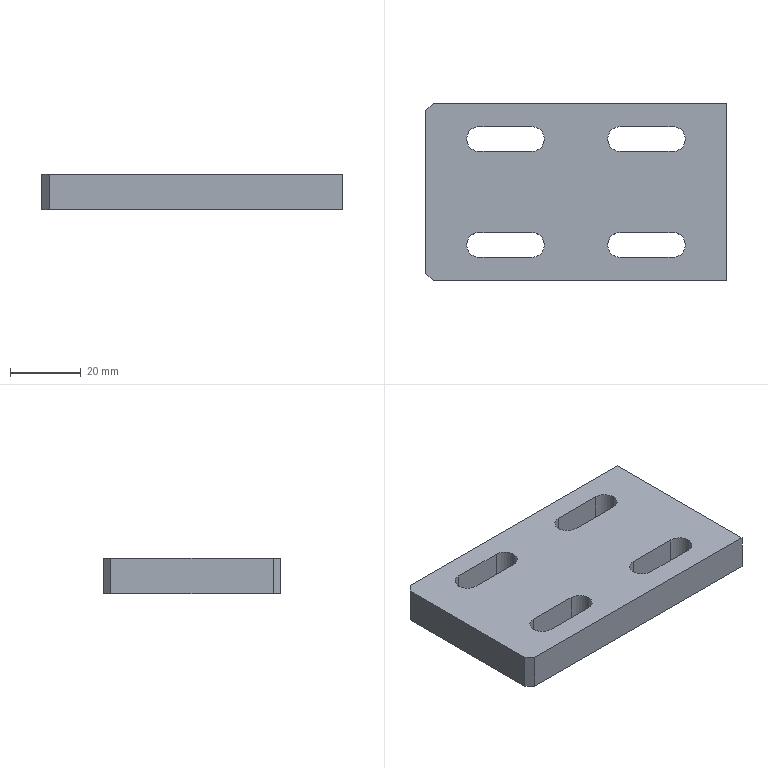Part | NX | 1 solid | 30 faces | box 85 x 50 x 10 mm | volume 36453 mm3 | plane 16 | cylinder 11 | cone 3 | commonest cylinder face diameters 7 x8 3.3 x3
STEP:
#1=CARTESIAN_POINT('',(-42.5,23.,-5.));
#2=VERTEX_POINT('',#1);
#3=CARTESIAN_POINT('',(-42.5,-23.,-5.));
#4=VERTEX_POINT('',#3);
#5=CARTESIAN_POINT('',(-42.5,-25.,-5.));
#6=DIRECTION('',(0.,-1.,0.));
#7=VECTOR('',#6,1000.);
#8=LINE('',#5,#7);
#9=EDGE_CURVE('',#2,#4,#8,.T.);
#10=ORIENTED_EDGE('',*,*,#9,.T.);
#11=CARTESIAN_POINT('',(-42.5,-23.,5.));
#12=VERTEX_POINT('',#11);
#13=CARTESIAN_POINT('',(-42.5,-23.,5.));
#14=DIRECTION('',(0.,0.,1.));
#15=VECTOR('',#14,1000.);
#16=LINE('',#13,#15);
#17=EDGE_CURVE('',#4,#12,#16,.T.);
#18=ORIENTED_EDGE('',*,*,#17,.T.);
#19=CARTESIAN_POINT('',(-42.5,23.,5.));
#20=VERTEX_POINT('',#19);
#21=CARTESIAN_POINT('',(-42.5,-25.,5.));
#22=DIRECTION('',(0.,-1.,0.));
#23=VECTOR('',#22,1000.);
#24=LINE('',#21,#23);
#25=EDGE_CURVE('',#20,#12,#24,.T.);
#26=ORIENTED_EDGE('',*,*,#25,.F.);
#27=CARTESIAN_POINT('',(-42.5,23.,5.));
#28=DIRECTION('',(0.,0.,-1.));
#29=VECTOR('',#28,1000.);
#30=LINE('',#27,#29);
#31=EDGE_CURVE('',#20,#2,#30,.T.);
#32=ORIENTED_EDGE('',*,*,#31,.T.);
#33=EDGE_LOOP('',(#10,#18,#26,#32));
#34=FACE_BOUND('',#33,.T.);
#35=CARTESIAN_POINT('',(-42.5,-25.,5.));
#36=DIRECTION('',(1.,0.,0.));
#37=DIRECTION('',(0.,0.,-1.));
#38=AXIS2_PLACEMENT_3D('',#35,#36,#37);
#39=PLANE('',#38);
#40=ADVANCED_FACE('',(#34),#39,.F.);
#41=CARTESIAN_POINT('',(-40.5,-25.,5.));
#42=VERTEX_POINT('',#41);
#43=CARTESIAN_POINT('',(42.5,-25.,5.));
#44=VERTEX_POINT('',#43);
#45=CARTESIAN_POINT('',(42.5,-25.,5.));
#46=DIRECTION('',(1.,0.,0.));
#47=VECTOR('',#46,1000.);
#48=LINE('',#45,#47);
#49=EDGE_CURVE('',#42,#44,#48,.T.);
#50=ORIENTED_EDGE('',*,*,#49,.F.);
#51=CARTESIAN_POINT('',(-40.5,-25.,-5.));
#52=VERTEX_POINT('',#51);
#53=CARTESIAN_POINT('',(-40.5,-25.,5.));
#54=DIRECTION('',(0.,0.,-1.));
#55=VECTOR('',#54,1000.);
#56=LINE('',#53,#55);
#57=EDGE_CURVE('',#42,#52,#56,.T.);
#58=ORIENTED_EDGE('',*,*,#57,.T.);
#59=CARTESIAN_POINT('',(42.5,-25.,-5.));
#60=VERTEX_POINT('',#59);
#61=CARTESIAN_POINT('',(42.5,-25.,-5.));
#62=DIRECTION('',(1.,0.,0.));
#63=VECTOR('',#62,1000.);
#64=LINE('',#61,#63);
#65=EDGE_CURVE('',#52,#60,#64,.T.);
#66=ORIENTED_EDGE('',*,*,#65,.T.);
#67=CARTESIAN_POINT('',(42.5,-25.,5.));
#68=DIRECTION('',(0.,0.,-1.));
#69=VECTOR('',#68,1000.);
#70=LINE('',#67,#69);
#71=EDGE_CURVE('',#44,#60,#70,.T.);
#72=ORIENTED_EDGE('',*,*,#71,.F.);
#73=EDGE_LOOP('',(#50,#58,#66,#72));
#74=FACE_BOUND('',#73,.T.);
#75=CARTESIAN_POINT('',(42.5,-25.,5.));
#76=DIRECTION('',(0.,1.,0.));
#77=DIRECTION('',(-1.,0.,0.));
#78=AXIS2_PLACEMENT_3D('',#75,#76,#77);
#79=PLANE('',#78);
#80=ADVANCED_FACE('',(#74),#79,.F.);
#81=CARTESIAN_POINT('',(42.5,17.5,-1.65));
#82=VERTEX_POINT('',#81);
#83=CARTESIAN_POINT('',(42.5,17.5,0.));
#84=DIRECTION('',(1.,0.,0.));
#85=DIRECTION('',(0.,0.,-1.));
#86=AXIS2_PLACEMENT_3D('',#83,#84,#85);
#87=CIRCLE('',#86,1.65);
#88=EDGE_CURVE('',#82,#82,#87,.T.);
#89=ORIENTED_EDGE('',*,*,#88,.F.);
#90=EDGE_LOOP('',(#89));
#91=FACE_BOUND('',#90,.T.);
#92=CARTESIAN_POINT('',(42.5,0.,-1.65));
#93=VERTEX_POINT('',#92);
#94=CARTESIAN_POINT('',(42.5,0.,0.));
#95=DIRECTION('',(1.,0.,0.));
#96=DIRECTION('',(0.,0.,-1.));
#97=AXIS2_PLACEMENT_3D('',#94,#95,#96);
#98=CIRCLE('',#97,1.65);
#99=EDGE_CURVE('',#93,#93,#98,.T.);
#100=ORIENTED_EDGE('',*,*,#99,.F.);
#101=EDGE_LOOP('',(#100));
#102=FACE_BOUND('',#101,.T.);
#103=CARTESIAN_POINT('',(42.5,-17.5,-1.65));
#104=VERTEX_POINT('',#103);
#105=CARTESIAN_POINT('',(42.5,-17.5,0.));
#106=DIRECTION('',(1.,0.,0.));
#107=DIRECTION('',(0.,0.,-1.));
#108=AXIS2_PLACEMENT_3D('',#105,#106,#107);
#109=CIRCLE('',#108,1.65);
#110=EDGE_CURVE('',#104,#104,#109,.T.);
#111=ORIENTED_EDGE('',*,*,#110,.F.);
#112=EDGE_LOOP('',(#111));
#113=FACE_BOUND('',#112,.T.);
#114=CARTESIAN_POINT('',(42.5,25.,-5.));
#115=VERTEX_POINT('',#114);
#116=CARTESIAN_POINT('',(42.5,-25.,-5.));
#117=DIRECTION('',(0.,1.,0.));
#118=VECTOR('',#117,1000.);
#119=LINE('',#116,#118);
#120=EDGE_CURVE('',#60,#115,#119,.T.);
#121=ORIENTED_EDGE('',*,*,#120,.T.);
#122=CARTESIAN_POINT('',(42.5,25.,5.));
#123=VERTEX_POINT('',#122);
#124=CARTESIAN_POINT('',(42.5,25.,5.));
#125=DIRECTION('',(0.,0.,-1.));
#126=VECTOR('',#125,1000.);
#127=LINE('',#124,#126);
#128=EDGE_CURVE('',#123,#115,#127,.T.);
#129=ORIENTED_EDGE('',*,*,#128,.F.);
#130=CARTESIAN_POINT('',(42.5,-25.,5.));
#131=DIRECTION('',(0.,1.,0.));
#132=VECTOR('',#131,1000.);
#133=LINE('',#130,#132);
#134=EDGE_CURVE('',#44,#123,#133,.T.);
#135=ORIENTED_EDGE('',*,*,#134,.F.);
#136=ORIENTED_EDGE('',*,*,#71,.T.);
#137=EDGE_LOOP('',(#121,#129,#135,#136));
#138=FACE_BOUND('',#137,.T.);
#139=CARTESIAN_POINT('',(42.5,-25.,5.));
#140=DIRECTION('',(-1.,0.,0.));
#141=DIRECTION('',(0.,0.,1.));
#142=AXIS2_PLACEMENT_3D('',#139,#140,#141);
#143=PLANE('',#142);
#144=ADVANCED_FACE('',(#91,#102,#113,#138),#143,.F.);
#145=CARTESIAN_POINT('',(-40.5,25.,-5.));
#146=VERTEX_POINT('',#145);
#147=CARTESIAN_POINT('',(42.5,25.,-5.));
#148=DIRECTION('',(-1.,0.,0.));
#149=VECTOR('',#148,1000.);
#150=LINE('',#147,#149);
#151=EDGE_CURVE('',#115,#146,#150,.T.);
#152=ORIENTED_EDGE('',*,*,#151,.T.);
#153=CARTESIAN_POINT('',(-40.5,25.,5.));
#154=VERTEX_POINT('',#153);
#155=CARTESIAN_POINT('',(-40.5,25.,5.));
#156=DIRECTION('',(0.,0.,1.));
#157=VECTOR('',#156,1000.);
#158=LINE('',#155,#157);
#159=EDGE_CURVE('',#146,#154,#158,.T.);
#160=ORIENTED_EDGE('',*,*,#159,.T.);
#161=CARTESIAN_POINT('',(42.5,25.,5.));
#162=DIRECTION('',(-1.,0.,0.));
#163=VECTOR('',#162,1000.);
#164=LINE('',#161,#163);
#165=EDGE_CURVE('',#123,#154,#164,.T.);
#166=ORIENTED_EDGE('',*,*,#165,.F.);
#167=ORIENTED_EDGE('',*,*,#128,.T.);
#168=EDGE_LOOP('',(#152,#160,#166,#167));
#169=FACE_BOUND('',#168,.T.);
#170=CARTESIAN_POINT('',(42.5,25.,5.));
#171=DIRECTION('',(0.,-1.,0.));
#172=DIRECTION('',(1.,0.,0.));
#173=AXIS2_PLACEMENT_3D('',#170,#171,#172);
#174=PLANE('',#173);
#175=ADVANCED_FACE('',(#169),#174,.F.);
#176=CARTESIAN_POINT('',(12.5,-11.5,5.));
#177=VERTEX_POINT('',#176);
#178=CARTESIAN_POINT('',(12.5,-18.5,5.));
#179=VERTEX_POINT('',#178);
#180=CARTESIAN_POINT('',(12.5,-15.,5.));
#181=DIRECTION('',(0.,0.,1.));
#182=DIRECTION('',(1.,0.,0.));
#183=AXIS2_PLACEMENT_3D('',#180,#181,#182);
#184=CIRCLE('',#183,3.5);
#185=EDGE_CURVE('',#177,#179,#184,.T.);
#186=ORIENTED_EDGE('',*,*,#185,.F.);
#187=CARTESIAN_POINT('',(27.5,-11.5,5.));
#188=VERTEX_POINT('',#187);
#189=CARTESIAN_POINT('',(12.5,-11.5,5.));
#190=DIRECTION('',(-1.,0.,0.));
#191=VECTOR('',#190,1000.);
#192=LINE('',#189,#191);
#193=EDGE_CURVE('',#188,#177,#192,.T.);
#194=ORIENTED_EDGE('',*,*,#193,.F.);
#195=CARTESIAN_POINT('',(27.5,-18.5,5.));
#196=VERTEX_POINT('',#195);
#197=CARTESIAN_POINT('',(27.5,-15.,5.));
#198=DIRECTION('',(0.,0.,1.));
#199=DIRECTION('',(1.,0.,0.));
#200=AXIS2_PLACEMENT_3D('',#197,#198,#199);
#201=CIRCLE('',#200,3.5);
#202=EDGE_CURVE('',#196,#188,#201,.T.);
#203=ORIENTED_EDGE('',*,*,#202,.F.);
#204=CARTESIAN_POINT('',(12.5,-18.5,5.));
#205=DIRECTION('',(1.,0.,0.));
#206=VECTOR('',#205,1000.);
#207=LINE('',#204,#206);
#208=EDGE_CURVE('',#179,#196,#207,.T.);
#209=ORIENTED_EDGE('',*,*,#208,.F.);
#210=EDGE_LOOP('',(#186,#194,#203,#209));
#211=FACE_BOUND('',#210,.T.);
#212=CARTESIAN_POINT('',(12.5,18.5,5.));
#213=VERTEX_POINT('',#212);
#214=CARTESIAN_POINT('',(12.5,11.5,5.));
#215=VERTEX_POINT('',#214);
#216=CARTESIAN_POINT('',(12.5,15.,5.));
#217=DIRECTION('',(0.,0.,1.));
#218=DIRECTION('',(1.,0.,0.));
#219=AXIS2_PLACEMENT_3D('',#216,#217,#218);
#220=CIRCLE('',#219,3.5);
#221=EDGE_CURVE('',#213,#215,#220,.T.);
#222=ORIENTED_EDGE('',*,*,#221,.F.);
#223=CARTESIAN_POINT('',(27.5,18.5,5.));
#224=VERTEX_POINT('',#223);
#225=CARTESIAN_POINT('',(12.5,18.5,5.));
#226=DIRECTION('',(-1.,0.,0.));
#227=VECTOR('',#226,1000.);
#228=LINE('',#225,#227);
#229=EDGE_CURVE('',#224,#213,#228,.T.);
#230=ORIENTED_EDGE('',*,*,#229,.F.);
#231=CARTESIAN_POINT('',(27.5,11.5,5.));
#232=VERTEX_POINT('',#231);
#233=CARTESIAN_POINT('',(27.5,15.,5.));
#234=DIRECTION('',(0.,0.,1.));
#235=DIRECTION('',(1.,0.,0.));
#236=AXIS2_PLACEMENT_3D('',#233,#234,#235);
#237=CIRCLE('',#236,3.5);
#238=EDGE_CURVE('',#232,#224,#237,.T.);
#239=ORIENTED_EDGE('',*,*,#238,.F.);
#240=CARTESIAN_POINT('',(12.5,11.5,5.));
#241=DIRECTION('',(1.,0.,0.));
#242=VECTOR('',#241,1000.);
#243=LINE('',#240,#242);
#244=EDGE_CURVE('',#215,#232,#243,.T.);
#245=ORIENTED_EDGE('',*,*,#244,.F.);
#246=EDGE_LOOP('',(#222,#230,#239,#245));
#247=FACE_BOUND('',#246,.T.);
#248=CARTESIAN_POINT('',(-27.5,-11.5,5.));
#249=VERTEX_POINT('',#248);
#250=CARTESIAN_POINT('',(-27.5,-18.5,5.));
#251=VERTEX_POINT('',#250);
#252=CARTESIAN_POINT('',(-27.5,-15.,5.));
#253=DIRECTION('',(0.,0.,1.));
#254=DIRECTION('',(1.,0.,0.));
#255=AXIS2_PLACEMENT_3D('',#252,#253,#254);
#256=CIRCLE('',#255,3.5);
#257=EDGE_CURVE('',#249,#251,#256,.T.);
#258=ORIENTED_EDGE('',*,*,#257,.F.);
#259=CARTESIAN_POINT('',(-12.5,-11.5,5.));
#260=VERTEX_POINT('',#259);
#261=CARTESIAN_POINT('',(-27.5,-11.5,5.));
#262=DIRECTION('',(-1.,0.,0.));
#263=VECTOR('',#262,1000.);
#264=LINE('',#261,#263);
#265=EDGE_CURVE('',#260,#249,#264,.T.);
#266=ORIENTED_EDGE('',*,*,#265,.F.);
#267=CARTESIAN_POINT('',(-12.5,-18.5,5.));
#268=VERTEX_POINT('',#267);
#269=CARTESIAN_POINT('',(-12.5,-15.,5.));
#270=DIRECTION('',(0.,0.,1.));
#271=DIRECTION('',(1.,0.,0.));
#272=AXIS2_PLACEMENT_3D('',#269,#270,#271);
#273=CIRCLE('',#272,3.5);
#274=EDGE_CURVE('',#268,#260,#273,.T.);
#275=ORIENTED_EDGE('',*,*,#274,.F.);
#276=CARTESIAN_POINT('',(-27.5,-18.5,5.));
#277=DIRECTION('',(1.,0.,0.));
#278=VECTOR('',#277,1000.);
#279=LINE('',#276,#278);
#280=EDGE_CURVE('',#251,#268,#279,.T.);
#281=ORIENTED_EDGE('',*,*,#280,.F.);
#282=EDGE_LOOP('',(#258,#266,#275,#281));
#283=FACE_BOUND('',#282,.T.);
#284=CARTESIAN_POINT('',(-27.5,18.5,5.));
#285=VERTEX_POINT('',#284);
#286=CARTESIAN_POINT('',(-27.5,11.5,5.));
#287=VERTEX_POINT('',#286);
#288=CARTESIAN_POINT('',(-27.5,15.,5.));
#289=DIRECTION('',(0.,0.,1.));
#290=DIRECTION('',(1.,0.,0.));
#291=AXIS2_PLACEMENT_3D('',#288,#289,#290);
#292=CIRCLE('',#291,3.5);
#293=EDGE_CURVE('',#285,#287,#292,.T.);
#294=ORIENTED_EDGE('',*,*,#293,.F.);
#295=CARTESIAN_POINT('',(-12.5,18.5,5.));
#296=VERTEX_POINT('',#295);
#297=CARTESIAN_POINT('',(-27.5,18.5,5.));
#298=DIRECTION('',(-1.,0.,0.));
#299=VECTOR('',#298,1000.);
#300=LINE('',#297,#299);
#301=EDGE_CURVE('',#296,#285,#300,.T.);
#302=ORIENTED_EDGE('',*,*,#301,.F.);
#303=CARTESIAN_POINT('',(-12.5,11.5,5.));
#304=VERTEX_POINT('',#303);
#305=CARTESIAN_POINT('',(-12.5,15.,5.));
#306=DIRECTION('',(0.,0.,1.));
#307=DIRECTION('',(1.,0.,0.));
#308=AXIS2_PLACEMENT_3D('',#305,#306,#307);
#309=CIRCLE('',#308,3.5);
#310=EDGE_CURVE('',#304,#296,#309,.T.);
#311=ORIENTED_EDGE('',*,*,#310,.F.);
#312=CARTESIAN_POINT('',(-27.5,11.5,5.));
#313=DIRECTION('',(1.,0.,0.));
#314=VECTOR('',#313,1000.);
#315=LINE('',#312,#314);
#316=EDGE_CURVE('',#287,#304,#315,.T.);
#317=ORIENTED_EDGE('',*,*,#316,.F.);
#318=EDGE_LOOP('',(#294,#302,#311,#317));
#319=FACE_BOUND('',#318,.T.);
#320=ORIENTED_EDGE('',*,*,#25,.T.);
#321=CARTESIAN_POINT('',(-32.75,-32.75,5.));
#322=DIRECTION('',(-0.7071,0.7071,0.));
#323=VECTOR('',#322,1000.);
#324=LINE('',#321,#323);
#325=EDGE_CURVE('',#12,#42,#324,.F.);
#326=ORIENTED_EDGE('',*,*,#325,.T.);
#327=ORIENTED_EDGE('',*,*,#49,.T.);
#328=ORIENTED_EDGE('',*,*,#134,.T.);
#329=ORIENTED_EDGE('',*,*,#165,.T.);
#330=CARTESIAN_POINT('',(-32.75,32.75,5.));
#331=DIRECTION('',(0.7071,0.7071,0.));
#332=VECTOR('',#331,1000.);
#333=LINE('',#330,#332);
#334=EDGE_CURVE('',#154,#20,#333,.F.);
#335=ORIENTED_EDGE('',*,*,#334,.T.);
#336=EDGE_LOOP('',(#320,#326,#327,#328,#329,#335));
#337=FACE_BOUND('',#336,.T.);
#338=CARTESIAN_POINT('',(0.,0.,5.));
#339=DIRECTION('',(0.,0.,1.));
#340=DIRECTION('',(1.,0.,0.));
#341=AXIS2_PLACEMENT_3D('',#338,#339,#340);
#342=PLANE('',#341);
#343=ADVANCED_FACE('',(#211,#247,#283,#319,#337),#342,.T.);
#344=CARTESIAN_POINT('',(27.5,-11.5,-5.));
#345=VERTEX_POINT('',#344);
#346=CARTESIAN_POINT('',(12.5,-11.5,-5.));
#347=VERTEX_POINT('',#346);
#348=CARTESIAN_POINT('',(12.5,-11.5,-5.));
#349=DIRECTION('',(-1.,0.,0.));
#350=VECTOR('',#349,1000.);
#351=LINE('',#348,#350);
#352=EDGE_CURVE('',#345,#347,#351,.T.);
#353=ORIENTED_EDGE('',*,*,#352,.T.);
#354=CARTESIAN_POINT('',(12.5,-18.5,-5.));
#355=VERTEX_POINT('',#354);
#356=CARTESIAN_POINT('',(12.5,-15.,-5.));
#357=DIRECTION('',(0.,0.,1.));
#358=DIRECTION('',(1.,0.,0.));
#359=AXIS2_PLACEMENT_3D('',#356,#357,#358);
#360=CIRCLE('',#359,3.5);
#361=EDGE_CURVE('',#347,#355,#360,.T.);
#362=ORIENTED_EDGE('',*,*,#361,.T.);
#363=CARTESIAN_POINT('',(27.5,-18.5,-5.));
#364=VERTEX_POINT('',#363);
#365=CARTESIAN_POINT('',(12.5,-18.5,-5.));
#366=DIRECTION('',(1.,0.,0.));
#367=VECTOR('',#366,1000.);
#368=LINE('',#365,#367);
#369=EDGE_CURVE('',#355,#364,#368,.T.);
#370=ORIENTED_EDGE('',*,*,#369,.T.);
#371=CARTESIAN_POINT('',(27.5,-15.,-5.));
#372=DIRECTION('',(0.,0.,1.));
#373=DIRECTION('',(1.,0.,0.));
#374=AXIS2_PLACEMENT_3D('',#371,#372,#373);
#375=CIRCLE('',#374,3.5);
#376=EDGE_CURVE('',#364,#345,#375,.T.);
#377=ORIENTED_EDGE('',*,*,#376,.T.);
#378=EDGE_LOOP('',(#353,#362,#370,#377));
#379=FACE_BOUND('',#378,.T.);
#380=CARTESIAN_POINT('',(27.5,18.5,-5.));
#381=VERTEX_POINT('',#380);
#382=CARTESIAN_POINT('',(12.5,18.5,-5.));
#383=VERTEX_POINT('',#382);
#384=CARTESIAN_POINT('',(12.5,18.5,-5.));
#385=DIRECTION('',(-1.,0.,0.));
#386=VECTOR('',#385,1000.);
#387=LINE('',#384,#386);
#388=EDGE_CURVE('',#381,#383,#387,.T.);
#389=ORIENTED_EDGE('',*,*,#388,.T.);
#390=CARTESIAN_POINT('',(12.5,11.5,-5.));
#391=VERTEX_POINT('',#390);
#392=CARTESIAN_POINT('',(12.5,15.,-5.));
#393=DIRECTION('',(0.,0.,1.));
#394=DIRECTION('',(1.,0.,0.));
#395=AXIS2_PLACEMENT_3D('',#392,#393,#394);
#396=CIRCLE('',#395,3.5);
#397=EDGE_CURVE('',#383,#391,#396,.T.);
#398=ORIENTED_EDGE('',*,*,#397,.T.);
#399=CARTESIAN_POINT('',(27.5,11.5,-5.));
#400=VERTEX_POINT('',#399);
#401=CARTESIAN_POINT('',(12.5,11.5,-5.));
#402=DIRECTION('',(1.,0.,0.));
#403=VECTOR('',#402,1000.);
#404=LINE('',#401,#403);
#405=EDGE_CURVE('',#391,#400,#404,.T.);
#406=ORIENTED_EDGE('',*,*,#405,.T.);
#407=CARTESIAN_POINT('',(27.5,15.,-5.));
#408=DIRECTION('',(0.,0.,1.));
#409=DIRECTION('',(1.,0.,0.));
#410=AXIS2_PLACEMENT_3D('',#407,#408,#409);
#411=CIRCLE('',#410,3.5);
#412=EDGE_CURVE('',#400,#381,#411,.T.);
#413=ORIENTED_EDGE('',*,*,#412,.T.);
#414=EDGE_LOOP('',(#389,#398,#406,#413));
#415=FACE_BOUND('',#414,.T.);
#416=CARTESIAN_POINT('',(-12.5,-11.5,-5.));
#417=VERTEX_POINT('',#416);
#418=CARTESIAN_POINT('',(-27.5,-11.5,-5.));
#419=VERTEX_POINT('',#418);
#420=CARTESIAN_POINT('',(-27.5,-11.5,-5.));
#421=DIRECTION('',(-1.,0.,0.));
#422=VECTOR('',#421,1000.);
#423=LINE('',#420,#422);
#424=EDGE_CURVE('',#417,#419,#423,.T.);
#425=ORIENTED_EDGE('',*,*,#424,.T.);
#426=CARTESIAN_POINT('',(-27.5,-18.5,-5.));
#427=VERTEX_POINT('',#426);
#428=CARTESIAN_POINT('',(-27.5,-15.,-5.));
#429=DIRECTION('',(0.,0.,1.));
#430=DIRECTION('',(1.,0.,0.));
#431=AXIS2_PLACEMENT_3D('',#428,#429,#430);
#432=CIRCLE('',#431,3.5);
#433=EDGE_CURVE('',#419,#427,#432,.T.);
#434=ORIENTED_EDGE('',*,*,#433,.T.);
#435=CARTESIAN_POINT('',(-12.5,-18.5,-5.));
#436=VERTEX_POINT('',#435);
#437=CARTESIAN_POINT('',(-27.5,-18.5,-5.));
#438=DIRECTION('',(1.,0.,0.));
#439=VECTOR('',#438,1000.);
#440=LINE('',#437,#439);
#441=EDGE_CURVE('',#427,#436,#440,.T.);
#442=ORIENTED_EDGE('',*,*,#441,.T.);
#443=CARTESIAN_POINT('',(-12.5,-15.,-5.));
#444=DIRECTION('',(0.,0.,1.));
#445=DIRECTION('',(1.,0.,0.));
#446=AXIS2_PLACEMENT_3D('',#443,#444,#445);
#447=CIRCLE('',#446,3.5);
#448=EDGE_CURVE('',#436,#417,#447,.T.);
#449=ORIENTED_EDGE('',*,*,#448,.T.);
#450=EDGE_LOOP('',(#425,#434,#442,#449));
#451=FACE_BOUND('',#450,.T.);
#452=CARTESIAN_POINT('',(-12.5,18.5,-5.));
#453=VERTEX_POINT('',#452);
#454=CARTESIAN_POINT('',(-27.5,18.5,-5.));
#455=VERTEX_POINT('',#454);
#456=CARTESIAN_POINT('',(-27.5,18.5,-5.));
#457=DIRECTION('',(-1.,0.,0.));
#458=VECTOR('',#457,1000.);
#459=LINE('',#456,#458);
#460=EDGE_CURVE('',#453,#455,#459,.T.);
#461=ORIENTED_EDGE('',*,*,#460,.T.);
#462=CARTESIAN_POINT('',(-27.5,11.5,-5.));
#463=VERTEX_POINT('',#462);
#464=CARTESIAN_POINT('',(-27.5,15.,-5.));
#465=DIRECTION('',(0.,0.,1.));
#466=DIRECTION('',(1.,0.,0.));
#467=AXIS2_PLACEMENT_3D('',#464,#465,#466);
#468=CIRCLE('',#467,3.5);
#469=EDGE_CURVE('',#455,#463,#468,.T.);
#470=ORIENTED_EDGE('',*,*,#469,.T.);
#471=CARTESIAN_POINT('',(-12.5,11.5,-5.));
#472=VERTEX_POINT('',#471);
#473=CARTESIAN_POINT('',(-27.5,11.5,-5.));
#474=DIRECTION('',(1.,0.,0.));
#475=VECTOR('',#474,1000.);
#476=LINE('',#473,#475);
#477=EDGE_CURVE('',#463,#472,#476,.T.);
#478=ORIENTED_EDGE('',*,*,#477,.T.);
#479=CARTESIAN_POINT('',(-12.5,15.,-5.));
#480=DIRECTION('',(0.,0.,1.));
#481=DIRECTION('',(1.,0.,0.));
#482=AXIS2_PLACEMENT_3D('',#479,#480,#481);
#483=CIRCLE('',#482,3.5);
#484=EDGE_CURVE('',#472,#453,#483,.T.);
#485=ORIENTED_EDGE('',*,*,#484,.T.);
#486=EDGE_LOOP('',(#461,#470,#478,#485));
#487=FACE_BOUND('',#486,.T.);
#488=ORIENTED_EDGE('',*,*,#65,.F.);
#489=CARTESIAN_POINT('',(-40.5,-25.,-5.));
#490=DIRECTION('',(0.7071,-0.7071,0.));
#491=VECTOR('',#490,1000.);
#492=LINE('',#489,#491);
#493=EDGE_CURVE('',#52,#4,#492,.F.);
#494=ORIENTED_EDGE('',*,*,#493,.T.);
#495=ORIENTED_EDGE('',*,*,#9,.F.);
#496=CARTESIAN_POINT('',(-42.5,23.,-5.));
#497=DIRECTION('',(-0.7071,-0.7071,0.));
#498=VECTOR('',#497,1000.);
#499=LINE('',#496,#498);
#500=EDGE_CURVE('',#2,#146,#499,.F.);
#501=ORIENTED_EDGE('',*,*,#500,.T.);
#502=ORIENTED_EDGE('',*,*,#151,.F.);
#503=ORIENTED_EDGE('',*,*,#120,.F.);
#504=EDGE_LOOP('',(#488,#494,#495,#501,#502,#503));
#505=FACE_BOUND('',#504,.T.);
#506=CARTESIAN_POINT('',(0.,0.,-5.));
#507=DIRECTION('',(0.,0.,1.));
#508=DIRECTION('',(1.,0.,0.));
#509=AXIS2_PLACEMENT_3D('',#506,#507,#508);
#510=PLANE('',#509);
#511=ADVANCED_FACE('',(#379,#415,#451,#487,#505),#510,.F.);
#512=ORIENTED_EDGE('',*,*,#293,.T.);
#513=CARTESIAN_POINT('',(-27.5,11.5,-5.));
#514=DIRECTION('',(0.,0.,1.));
#515=VECTOR('',#514,1000.);
#516=LINE('',#513,#515);
#517=EDGE_CURVE('',#463,#287,#516,.T.);
#518=ORIENTED_EDGE('',*,*,#517,.F.);
#519=ORIENTED_EDGE('',*,*,#469,.F.);
#520=CARTESIAN_POINT('',(-27.5,18.5,-5.));
#521=DIRECTION('',(0.,0.,1.));
#522=VECTOR('',#521,1000.);
#523=LINE('',#520,#522);
#524=EDGE_CURVE('',#455,#285,#523,.T.);
#525=ORIENTED_EDGE('',*,*,#524,.T.);
#526=EDGE_LOOP('',(#512,#518,#519,#525));
#527=FACE_BOUND('',#526,.T.);
#528=CARTESIAN_POINT('',(-27.5,15.,-5.));
#529=DIRECTION('',(0.,0.,1.));
#530=DIRECTION('',(1.,0.,0.));
#531=AXIS2_PLACEMENT_3D('',#528,#529,#530);
#532=CYLINDRICAL_SURFACE('',#531,3.5);
#533=ADVANCED_FACE('',(#527),#532,.F.);
#534=ORIENTED_EDGE('',*,*,#301,.T.);
#535=ORIENTED_EDGE('',*,*,#524,.F.);
#536=ORIENTED_EDGE('',*,*,#460,.F.);
#537=CARTESIAN_POINT('',(-12.5,18.5,-5.));
#538=DIRECTION('',(0.,0.,1.));
#539=VECTOR('',#538,1000.);
#540=LINE('',#537,#539);
#541=EDGE_CURVE('',#453,#296,#540,.T.);
#542=ORIENTED_EDGE('',*,*,#541,.T.);
#543=EDGE_LOOP('',(#534,#535,#536,#542));
#544=FACE_BOUND('',#543,.T.);
#545=CARTESIAN_POINT('',(-27.5,18.5,-5.));
#546=DIRECTION('',(0.,1.,0.));
#547=DIRECTION('',(-1.,0.,0.));
#548=AXIS2_PLACEMENT_3D('',#545,#546,#547);
#549=PLANE('',#548);
#550=ADVANCED_FACE('',(#544),#549,.F.);
#551=ORIENTED_EDGE('',*,*,#310,.T.);
#552=ORIENTED_EDGE('',*,*,#541,.F.);
#553=ORIENTED_EDGE('',*,*,#484,.F.);
#554=CARTESIAN_POINT('',(-12.5,11.5,-5.));
#555=DIRECTION('',(0.,0.,1.));
#556=VECTOR('',#555,1000.);
#557=LINE('',#554,#556);
#558=EDGE_CURVE('',#472,#304,#557,.T.);
#559=ORIENTED_EDGE('',*,*,#558,.T.);
#560=EDGE_LOOP('',(#551,#552,#553,#559));
#561=FACE_BOUND('',#560,.T.);
#562=CARTESIAN_POINT('',(-12.5,15.,-5.));
#563=DIRECTION('',(0.,0.,1.));
#564=DIRECTION('',(1.,0.,0.));
#565=AXIS2_PLACEMENT_3D('',#562,#563,#564);
#566=CYLINDRICAL_SURFACE('',#565,3.5);
#567=ADVANCED_FACE('',(#561),#566,.F.);
#568=ORIENTED_EDGE('',*,*,#316,.T.);
#569=ORIENTED_EDGE('',*,*,#558,.F.);
#570=ORIENTED_EDGE('',*,*,#477,.F.);
#571=ORIENTED_EDGE('',*,*,#517,.T.);
#572=EDGE_LOOP('',(#568,#569,#570,#571));
#573=FACE_BOUND('',#572,.T.);
#574=CARTESIAN_POINT('',(-27.5,11.5,-5.));
#575=DIRECTION('',(0.,-1.,0.));
#576=DIRECTION('',(1.,0.,0.));
#577=AXIS2_PLACEMENT_3D('',#574,#575,#576);
#578=PLANE('',#577);
#579=ADVANCED_FACE('',(#573),#578,.F.);
#580=ORIENTED_EDGE('',*,*,#257,.T.);
#581=CARTESIAN_POINT('',(-27.5,-18.5,-5.));
#582=DIRECTION('',(0.,0.,1.));
#583=VECTOR('',#582,1000.);
#584=LINE('',#581,#583);
#585=EDGE_CURVE('',#427,#251,#584,.T.);
#586=ORIENTED_EDGE('',*,*,#585,.F.);
#587=ORIENTED_EDGE('',*,*,#433,.F.);
#588=CARTESIAN_POINT('',(-27.5,-11.5,-5.));
#589=DIRECTION('',(0.,0.,1.));
#590=VECTOR('',#589,1000.);
#591=LINE('',#588,#590);
#592=EDGE_CURVE('',#419,#249,#591,.T.);
#593=ORIENTED_EDGE('',*,*,#592,.T.);
#594=EDGE_LOOP('',(#580,#586,#587,#593));
#595=FACE_BOUND('',#594,.T.);
#596=CARTESIAN_POINT('',(-27.5,-15.,-5.));
#597=DIRECTION('',(0.,0.,1.));
#598=DIRECTION('',(1.,0.,0.));
#599=AXIS2_PLACEMENT_3D('',#596,#597,#598);
#600=CYLINDRICAL_SURFACE('',#599,3.5);
#601=ADVANCED_FACE('',(#595),#600,.F.);
#602=ORIENTED_EDGE('',*,*,#265,.T.);
#603=ORIENTED_EDGE('',*,*,#592,.F.);
#604=ORIENTED_EDGE('',*,*,#424,.F.);
#605=CARTESIAN_POINT('',(-12.5,-11.5,-5.));
#606=DIRECTION('',(0.,0.,1.));
#607=VECTOR('',#606,1000.);
#608=LINE('',#605,#607);
#609=EDGE_CURVE('',#417,#260,#608,.T.);
#610=ORIENTED_EDGE('',*,*,#609,.T.);
#611=EDGE_LOOP('',(#602,#603,#604,#610));
#612=FACE_BOUND('',#611,.T.);
#613=CARTESIAN_POINT('',(-27.5,-11.5,-5.));
#614=DIRECTION('',(0.,1.,0.));
#615=DIRECTION('',(-1.,0.,0.));
#616=AXIS2_PLACEMENT_3D('',#613,#614,#615);
#617=PLANE('',#616);
#618=ADVANCED_FACE('',(#612),#617,.F.);
#619=ORIENTED_EDGE('',*,*,#274,.T.);
#620=ORIENTED_EDGE('',*,*,#609,.F.);
#621=ORIENTED_EDGE('',*,*,#448,.F.);
#622=CARTESIAN_POINT('',(-12.5,-18.5,-5.));
#623=DIRECTION('',(0.,0.,1.));
#624=VECTOR('',#623,1000.);
#625=LINE('',#622,#624);
#626=EDGE_CURVE('',#436,#268,#625,.T.);
#627=ORIENTED_EDGE('',*,*,#626,.T.);
#628=EDGE_LOOP('',(#619,#620,#621,#627));
#629=FACE_BOUND('',#628,.T.);
#630=CARTESIAN_POINT('',(-12.5,-15.,-5.));
#631=DIRECTION('',(0.,0.,1.));
#632=DIRECTION('',(1.,0.,0.));
#633=AXIS2_PLACEMENT_3D('',#630,#631,#632);
#634=CYLINDRICAL_SURFACE('',#633,3.5);
#635=ADVANCED_FACE('',(#629),#634,.F.);
#636=ORIENTED_EDGE('',*,*,#280,.T.);
#637=ORIENTED_EDGE('',*,*,#626,.F.);
#638=ORIENTED_EDGE('',*,*,#441,.F.);
#639=ORIENTED_EDGE('',*,*,#585,.T.);
#640=EDGE_LOOP('',(#636,#637,#638,#639));
#641=FACE_BOUND('',#640,.T.);
#642=CARTESIAN_POINT('',(-27.5,-18.5,-5.));
#643=DIRECTION('',(0.,-1.,0.));
#644=DIRECTION('',(1.,0.,0.));
#645=AXIS2_PLACEMENT_3D('',#642,#643,#644);
#646=PLANE('',#645);
#647=ADVANCED_FACE('',(#641),#646,.F.);
#648=CARTESIAN_POINT('',(31.409,-17.5,0.));
#649=VERTEX_POINT('',#648);
#650=VERTEX_LOOP('',#649);
#651=FACE_BOUND('',#650,.T.);
#652=CARTESIAN_POINT('',(32.4,-17.5,-1.65));
#653=VERTEX_POINT('',#652);
#654=CARTESIAN_POINT('',(32.4,-17.5,0.));
#655=DIRECTION('',(1.,0.,0.));
#656=DIRECTION('',(0.,0.,-1.));
#657=AXIS2_PLACEMENT_3D('',#654,#655,#656);
#658=CIRCLE('',#657,1.65);
#659=EDGE_CURVE('',#653,#653,#658,.T.);
#660=ORIENTED_EDGE('',*,*,#659,.T.);
#661=EDGE_LOOP('',(#660));
#662=FACE_BOUND('',#661,.T.);
#663=CARTESIAN_POINT('',(32.4,-17.5,0.));
#664=DIRECTION('',(1.,0.,0.));
#665=DIRECTION('',(0.,0.,-1.));
#666=AXIS2_PLACEMENT_3D('',#663,#664,#665);
#667=CONICAL_SURFACE('',#666,1.65,1.03);
#668=ADVANCED_FACE('',(#651,#662),#667,.F.);
#669=ORIENTED_EDGE('',*,*,#659,.F.);
#670=EDGE_LOOP('',(#669));
#671=FACE_BOUND('',#670,.T.);
#672=ORIENTED_EDGE('',*,*,#110,.T.);
#673=EDGE_LOOP('',(#672));
#674=FACE_BOUND('',#673,.T.);
#675=CARTESIAN_POINT('',(42.5,-17.5,0.));
#676=DIRECTION('',(1.,0.,0.));
#677=DIRECTION('',(0.,0.,-1.));
#678=AXIS2_PLACEMENT_3D('',#675,#676,#677);
#679=CYLINDRICAL_SURFACE('',#678,1.65);
#680=ADVANCED_FACE('',(#671,#674),#679,.F.);
#681=CARTESIAN_POINT('',(31.409,0.,0.));
#682=VERTEX_POINT('',#681);
#683=VERTEX_LOOP('',#682);
#684=FACE_BOUND('',#683,.T.);
#685=CARTESIAN_POINT('',(32.4,0.,-1.65));
#686=VERTEX_POINT('',#685);
#687=CARTESIAN_POINT('',(32.4,0.,0.));
#688=DIRECTION('',(1.,0.,0.));
#689=DIRECTION('',(0.,0.,-1.));
#690=AXIS2_PLACEMENT_3D('',#687,#688,#689);
#691=CIRCLE('',#690,1.65);
#692=EDGE_CURVE('',#686,#686,#691,.T.);
#693=ORIENTED_EDGE('',*,*,#692,.T.);
#694=EDGE_LOOP('',(#693));
#695=FACE_BOUND('',#694,.T.);
#696=CARTESIAN_POINT('',(32.4,0.,0.));
#697=DIRECTION('',(1.,0.,0.));
#698=DIRECTION('',(0.,0.,-1.));
#699=AXIS2_PLACEMENT_3D('',#696,#697,#698);
#700=CONICAL_SURFACE('',#699,1.65,1.03);
#701=ADVANCED_FACE('',(#684,#695),#700,.F.);
#702=ORIENTED_EDGE('',*,*,#692,.F.);
#703=EDGE_LOOP('',(#702));
#704=FACE_BOUND('',#703,.T.);
#705=ORIENTED_EDGE('',*,*,#99,.T.);
#706=EDGE_LOOP('',(#705));
#707=FACE_BOUND('',#706,.T.);
#708=CARTESIAN_POINT('',(42.5,0.,0.));
#709=DIRECTION('',(1.,0.,0.));
#710=DIRECTION('',(0.,0.,-1.));
#711=AXIS2_PLACEMENT_3D('',#708,#709,#710);
#712=CYLINDRICAL_SURFACE('',#711,1.65);
#713=ADVANCED_FACE('',(#704,#707),#712,.F.);
#714=CARTESIAN_POINT('',(31.409,17.5,0.));
#715=VERTEX_POINT('',#714);
#716=VERTEX_LOOP('',#715);
#717=FACE_BOUND('',#716,.T.);
#718=CARTESIAN_POINT('',(32.4,17.5,-1.65));
#719=VERTEX_POINT('',#718);
#720=CARTESIAN_POINT('',(32.4,17.5,0.));
#721=DIRECTION('',(1.,0.,0.));
#722=DIRECTION('',(0.,0.,-1.));
#723=AXIS2_PLACEMENT_3D('',#720,#721,#722);
#724=CIRCLE('',#723,1.65);
#725=EDGE_CURVE('',#719,#719,#724,.T.);
#726=ORIENTED_EDGE('',*,*,#725,.T.);
#727=EDGE_LOOP('',(#726));
#728=FACE_BOUND('',#727,.T.);
#729=CARTESIAN_POINT('',(32.4,17.5,0.));
#730=DIRECTION('',(1.,0.,0.));
#731=DIRECTION('',(0.,0.,-1.));
#732=AXIS2_PLACEMENT_3D('',#729,#730,#731);
#733=CONICAL_SURFACE('',#732,1.65,1.03);
#734=ADVANCED_FACE('',(#717,#728),#733,.F.);
#735=ORIENTED_EDGE('',*,*,#725,.F.);
#736=EDGE_LOOP('',(#735));
#737=FACE_BOUND('',#736,.T.);
#738=ORIENTED_EDGE('',*,*,#88,.T.);
#739=EDGE_LOOP('',(#738));
#740=FACE_BOUND('',#739,.T.);
#741=CARTESIAN_POINT('',(42.5,17.5,0.));
#742=DIRECTION('',(1.,0.,0.));
#743=DIRECTION('',(0.,0.,-1.));
#744=AXIS2_PLACEMENT_3D('',#741,#742,#743);
#745=CYLINDRICAL_SURFACE('',#744,1.65);
#746=ADVANCED_FACE('',(#737,#740),#745,.F.);
#747=ORIENTED_EDGE('',*,*,#325,.F.);
#748=ORIENTED_EDGE('',*,*,#17,.F.);
#749=ORIENTED_EDGE('',*,*,#493,.F.);
#750=ORIENTED_EDGE('',*,*,#57,.F.);
#751=EDGE_LOOP('',(#747,#748,#749,#750));
#752=FACE_BOUND('',#751,.T.);
#753=CARTESIAN_POINT('',(-40.5,-25.,5.));
#754=DIRECTION('',(0.7071,0.7071,0.));
#755=DIRECTION('',(0.,0.,-1.));
#756=AXIS2_PLACEMENT_3D('',#753,#754,#755);
#757=PLANE('',#756);
#758=ADVANCED_FACE('',(#752),#757,.F.);
#759=ORIENTED_EDGE('',*,*,#334,.F.);
#760=ORIENTED_EDGE('',*,*,#159,.F.);
#761=ORIENTED_EDGE('',*,*,#500,.F.);
#762=ORIENTED_EDGE('',*,*,#31,.F.);
#763=EDGE_LOOP('',(#759,#760,#761,#762));
#764=FACE_BOUND('',#763,.T.);
#765=CARTESIAN_POINT('',(-42.5,23.,5.));
#766=DIRECTION('',(0.7071,-0.7071,0.));
#767=DIRECTION('',(0.,0.,-1.));
#768=AXIS2_PLACEMENT_3D('',#765,#766,#767);
#769=PLANE('',#768);
#770=ADVANCED_FACE('',(#764),#769,.F.);
#771=ORIENTED_EDGE('',*,*,#221,.T.);
#772=CARTESIAN_POINT('',(12.5,11.5,-5.));
#773=DIRECTION('',(0.,0.,1.));
#774=VECTOR('',#773,1000.);
#775=LINE('',#772,#774);
#776=EDGE_CURVE('',#391,#215,#775,.T.);
#777=ORIENTED_EDGE('',*,*,#776,.F.);
#778=ORIENTED_EDGE('',*,*,#397,.F.);
#779=CARTESIAN_POINT('',(12.5,18.5,-5.));
#780=DIRECTION('',(0.,0.,1.));
#781=VECTOR('',#780,1000.);
#782=LINE('',#779,#781);
#783=EDGE_CURVE('',#383,#213,#782,.T.);
#784=ORIENTED_EDGE('',*,*,#783,.T.);
#785=EDGE_LOOP('',(#771,#777,#778,#784));
#786=FACE_BOUND('',#785,.T.);
#787=CARTESIAN_POINT('',(12.5,15.,-5.));
#788=DIRECTION('',(0.,0.,1.));
#789=DIRECTION('',(1.,0.,0.));
#790=AXIS2_PLACEMENT_3D('',#787,#788,#789);
#791=CYLINDRICAL_SURFACE('',#790,3.5);
#792=ADVANCED_FACE('',(#786),#791,.F.);
#793=ORIENTED_EDGE('',*,*,#229,.T.);
#794=ORIENTED_EDGE('',*,*,#783,.F.);
#795=ORIENTED_EDGE('',*,*,#388,.F.);
#796=CARTESIAN_POINT('',(27.5,18.5,-5.));
#797=DIRECTION('',(0.,0.,1.));
#798=VECTOR('',#797,1000.);
#799=LINE('',#796,#798);
#800=EDGE_CURVE('',#381,#224,#799,.T.);
#801=ORIENTED_EDGE('',*,*,#800,.T.);
#802=EDGE_LOOP('',(#793,#794,#795,#801));
#803=FACE_BOUND('',#802,.T.);
#804=CARTESIAN_POINT('',(12.5,18.5,-5.));
#805=DIRECTION('',(0.,1.,0.));
#806=DIRECTION('',(-1.,0.,0.));
#807=AXIS2_PLACEMENT_3D('',#804,#805,#806);
#808=PLANE('',#807);
#809=ADVANCED_FACE('',(#803),#808,.F.);
#810=ORIENTED_EDGE('',*,*,#238,.T.);
#811=ORIENTED_EDGE('',*,*,#800,.F.);
#812=ORIENTED_EDGE('',*,*,#412,.F.);
#813=CARTESIAN_POINT('',(27.5,11.5,-5.));
#814=DIRECTION('',(0.,0.,1.));
#815=VECTOR('',#814,1000.);
#816=LINE('',#813,#815);
#817=EDGE_CURVE('',#400,#232,#816,.T.);
#818=ORIENTED_EDGE('',*,*,#817,.T.);
#819=EDGE_LOOP('',(#810,#811,#812,#818));
#820=FACE_BOUND('',#819,.T.);
#821=CARTESIAN_POINT('',(27.5,15.,-5.));
#822=DIRECTION('',(0.,0.,1.));
#823=DIRECTION('',(1.,0.,0.));
#824=AXIS2_PLACEMENT_3D('',#821,#822,#823);
#825=CYLINDRICAL_SURFACE('',#824,3.5);
#826=ADVANCED_FACE('',(#820),#825,.F.);
#827=ORIENTED_EDGE('',*,*,#244,.T.);
#828=ORIENTED_EDGE('',*,*,#817,.F.);
#829=ORIENTED_EDGE('',*,*,#405,.F.);
#830=ORIENTED_EDGE('',*,*,#776,.T.);
#831=EDGE_LOOP('',(#827,#828,#829,#830));
#832=FACE_BOUND('',#831,.T.);
#833=CARTESIAN_POINT('',(12.5,11.5,-5.));
#834=DIRECTION('',(0.,-1.,0.));
#835=DIRECTION('',(1.,0.,0.));
#836=AXIS2_PLACEMENT_3D('',#833,#834,#835);
#837=PLANE('',#836);
#838=ADVANCED_FACE('',(#832),#837,.F.);
#839=ORIENTED_EDGE('',*,*,#185,.T.);
#840=CARTESIAN_POINT('',(12.5,-18.5,-5.));
#841=DIRECTION('',(0.,0.,1.));
#842=VECTOR('',#841,1000.);
#843=LINE('',#840,#842);
#844=EDGE_CURVE('',#355,#179,#843,.T.);
#845=ORIENTED_EDGE('',*,*,#844,.F.);
#846=ORIENTED_EDGE('',*,*,#361,.F.);
#847=CARTESIAN_POINT('',(12.5,-11.5,-5.));
#848=DIRECTION('',(0.,0.,1.));
#849=VECTOR('',#848,1000.);
#850=LINE('',#847,#849);
#851=EDGE_CURVE('',#347,#177,#850,.T.);
#852=ORIENTED_EDGE('',*,*,#851,.T.);
#853=EDGE_LOOP('',(#839,#845,#846,#852));
#854=FACE_BOUND('',#853,.T.);
#855=CARTESIAN_POINT('',(12.5,-15.,-5.));
#856=DIRECTION('',(0.,0.,1.));
#857=DIRECTION('',(1.,0.,0.));
#858=AXIS2_PLACEMENT_3D('',#855,#856,#857);
#859=CYLINDRICAL_SURFACE('',#858,3.5);
#860=ADVANCED_FACE('',(#854),#859,.F.);
#861=ORIENTED_EDGE('',*,*,#193,.T.);
#862=ORIENTED_EDGE('',*,*,#851,.F.);
#863=ORIENTED_EDGE('',*,*,#352,.F.);
#864=CARTESIAN_POINT('',(27.5,-11.5,-5.));
#865=DIRECTION('',(0.,0.,1.));
#866=VECTOR('',#865,1000.);
#867=LINE('',#864,#866);
#868=EDGE_CURVE('',#345,#188,#867,.T.);
#869=ORIENTED_EDGE('',*,*,#868,.T.);
#870=EDGE_LOOP('',(#861,#862,#863,#869));
#871=FACE_BOUND('',#870,.T.);
#872=CARTESIAN_POINT('',(12.5,-11.5,-5.));
#873=DIRECTION('',(0.,1.,0.));
#874=DIRECTION('',(-1.,0.,0.));
#875=AXIS2_PLACEMENT_3D('',#872,#873,#874);
#876=PLANE('',#875);
#877=ADVANCED_FACE('',(#871),#876,.F.);
#878=ORIENTED_EDGE('',*,*,#202,.T.);
#879=ORIENTED_EDGE('',*,*,#868,.F.);
#880=ORIENTED_EDGE('',*,*,#376,.F.);
#881=CARTESIAN_POINT('',(27.5,-18.5,-5.));
#882=DIRECTION('',(0.,0.,1.));
#883=VECTOR('',#882,1000.);
#884=LINE('',#881,#883);
#885=EDGE_CURVE('',#364,#196,#884,.T.);
#886=ORIENTED_EDGE('',*,*,#885,.T.);
#887=EDGE_LOOP('',(#878,#879,#880,#886));
#888=FACE_BOUND('',#887,.T.);
#889=CARTESIAN_POINT('',(27.5,-15.,-5.));
#890=DIRECTION('',(0.,0.,1.));
#891=DIRECTION('',(1.,0.,0.));
#892=AXIS2_PLACEMENT_3D('',#889,#890,#891);
#893=CYLINDRICAL_SURFACE('',#892,3.5);
#894=ADVANCED_FACE('',(#888),#893,.F.);
#895=ORIENTED_EDGE('',*,*,#208,.T.);
#896=ORIENTED_EDGE('',*,*,#885,.F.);
#897=ORIENTED_EDGE('',*,*,#369,.F.);
#898=ORIENTED_EDGE('',*,*,#844,.T.);
#899=EDGE_LOOP('',(#895,#896,#897,#898));
#900=FACE_BOUND('',#899,.T.);
#901=CARTESIAN_POINT('',(12.5,-18.5,-5.));
#902=DIRECTION('',(0.,-1.,0.));
#903=DIRECTION('',(1.,0.,0.));
#904=AXIS2_PLACEMENT_3D('',#901,#902,#903);
#905=PLANE('',#904);
#906=ADVANCED_FACE('',(#900),#905,.F.);
#907=CLOSED_SHELL('',(#40,#80,#144,#175,#343,#511,#533,#550,#567,#579,#601,#618,#635,#647,#668,#680,#701,#713,#734,#746,#758,#770,#792,#809,#826,#838,#860,#877,#894,#906));
#908=MANIFOLD_SOLID_BREP('',#907);
#909=(LENGTH_UNIT()NAMED_UNIT(*)SI_UNIT(.MILLI.,.METRE.));
#910=UNCERTAINTY_MEASURE_WITH_UNIT(LENGTH_MEASURE(0.00001),#909,'','');
#911=(NAMED_UNIT(*)PLANE_ANGLE_UNIT()SI_UNIT($,.RADIAN.));
#912=(NAMED_UNIT(*)SI_UNIT($,.STERADIAN.)SOLID_ANGLE_UNIT());
#913=(GEOMETRIC_REPRESENTATION_CONTEXT(3)GLOBAL_UNCERTAINTY_ASSIGNED_CONTEXT((#910))GLOBAL_UNIT_ASSIGNED_CONTEXT((#909,#911,#912))REPRESENTATION_CONTEXT('',''));
#914=ADVANCED_BREP_SHAPE_REPRESENTATION('',(#908),#913);